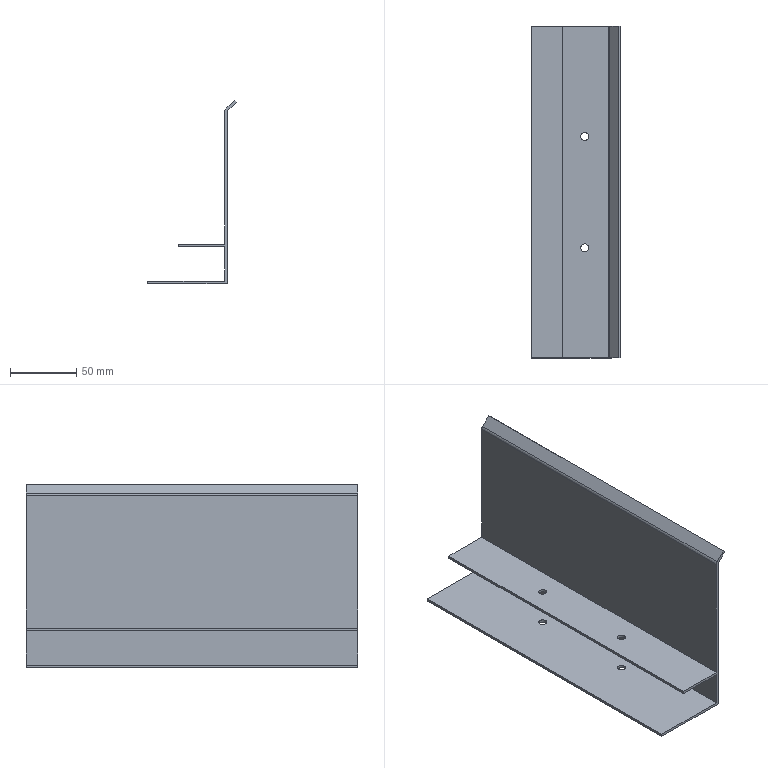Part | STEP file | zheshangyeban | 1 solid | 20 faces | box 67 x 250 x 138.414 mm | volume 116601 mm3 | plane 14 | cylinder 6 | commonest cylinder face diameters 6 x5 3 x1